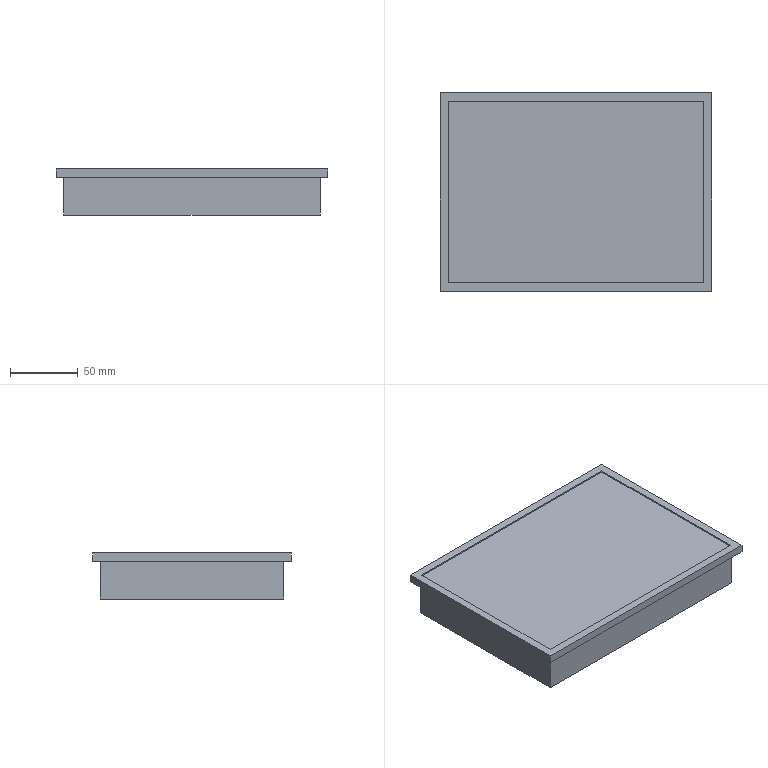Part | SolidWorks | features ICE 2, Extrusion 1 | 1 solid | 16 faces | box 200.3 x 146.3 x 34 mm | volume 870408 mm3 | plane 16
STEP:
#1=CARTESIAN_POINT('',(100.15,-73.15,0.));
#2=VERTEX_POINT('',#1);
#3=CARTESIAN_POINT('',(100.15,73.15,0.));
#4=VERTEX_POINT('',#3);
#5=CARTESIAN_POINT('',(100.15,73.15,0.));
#6=DIRECTION('',(0.,1.,0.));
#7=VECTOR('',#6,1000.);
#8=LINE('',#5,#7);
#9=EDGE_CURVE('',#2,#4,#8,.T.);
#10=ORIENTED_EDGE('',*,*,#9,.F.);
#11=CARTESIAN_POINT('',(-100.15,-73.15,0.));
#12=VERTEX_POINT('',#11);
#13=CARTESIAN_POINT('',(-100.15,-73.15,0.));
#14=DIRECTION('',(1.,0.,0.));
#15=VECTOR('',#14,1000.);
#16=LINE('',#13,#15);
#17=EDGE_CURVE('',#12,#2,#16,.T.);
#18=ORIENTED_EDGE('',*,*,#17,.F.);
#19=CARTESIAN_POINT('',(-100.15,73.15,0.));
#20=VERTEX_POINT('',#19);
#21=CARTESIAN_POINT('',(-100.15,73.15,0.));
#22=DIRECTION('',(0.,-1.,0.));
#23=VECTOR('',#22,1000.);
#24=LINE('',#21,#23);
#25=EDGE_CURVE('',#20,#12,#24,.T.);
#26=ORIENTED_EDGE('',*,*,#25,.F.);
#27=CARTESIAN_POINT('',(-100.15,73.15,0.));
#28=DIRECTION('',(-1.,0.,0.));
#29=VECTOR('',#28,1000.);
#30=LINE('',#27,#29);
#31=EDGE_CURVE('',#4,#20,#30,.T.);
#32=ORIENTED_EDGE('',*,*,#31,.F.);
#33=EDGE_LOOP('',(#10,#18,#26,#32));
#34=FACE_OUTER_BOUND('',#33,.T.);
#35=CARTESIAN_POINT('',(-94.8,-67.8,0.));
#36=VERTEX_POINT('',#35);
#37=CARTESIAN_POINT('',(-94.8,67.8,0.));
#38=VERTEX_POINT('',#37);
#39=CARTESIAN_POINT('',(-94.8,67.8,0.));
#40=DIRECTION('',(0.,1.,0.));
#41=VECTOR('',#40,1000.);
#42=LINE('',#39,#41);
#43=EDGE_CURVE('',#36,#38,#42,.T.);
#44=ORIENTED_EDGE('',*,*,#43,.F.);
#45=CARTESIAN_POINT('',(94.8,-67.8,0.));
#46=VERTEX_POINT('',#45);
#47=CARTESIAN_POINT('',(94.8,-67.8,0.));
#48=DIRECTION('',(-1.,0.,0.));
#49=VECTOR('',#48,1000.);
#50=LINE('',#47,#49);
#51=EDGE_CURVE('',#46,#36,#50,.T.);
#52=ORIENTED_EDGE('',*,*,#51,.F.);
#53=CARTESIAN_POINT('',(94.8,67.8,0.));
#54=VERTEX_POINT('',#53);
#55=CARTESIAN_POINT('',(94.8,67.8,0.));
#56=DIRECTION('',(0.,-1.,0.));
#57=VECTOR('',#56,1000.);
#58=LINE('',#55,#57);
#59=EDGE_CURVE('',#54,#46,#58,.T.);
#60=ORIENTED_EDGE('',*,*,#59,.F.);
#61=CARTESIAN_POINT('',(94.8,67.8,0.));
#62=DIRECTION('',(1.,0.,0.));
#63=VECTOR('',#62,1000.);
#64=LINE('',#61,#63);
#65=EDGE_CURVE('',#38,#54,#64,.T.);
#66=ORIENTED_EDGE('',*,*,#65,.F.);
#67=EDGE_LOOP('',(#44,#52,#60,#66));
#68=FACE_BOUND('',#67,.T.);
#69=CARTESIAN_POINT('',(0.,0.,0.));
#70=DIRECTION('',(0.,0.,1.));
#71=DIRECTION('',(1.,0.,0.));
#72=AXIS2_PLACEMENT_3D('',#69,#70,#71);
#73=PLANE('',#72);
#74=ADVANCED_FACE('',(#34,#68),#73,.F.);
#75=ORIENTED_EDGE('',*,*,#9,.T.);
#76=CARTESIAN_POINT('',(100.15,73.15,6.));
#77=VERTEX_POINT('',#76);
#78=CARTESIAN_POINT('',(100.15,73.15,6.));
#79=DIRECTION('',(0.,0.,-1.));
#80=VECTOR('',#79,1000.);
#81=LINE('',#78,#80);
#82=EDGE_CURVE('',#77,#4,#81,.T.);
#83=ORIENTED_EDGE('',*,*,#82,.F.);
#84=CARTESIAN_POINT('',(100.15,-73.15,6.));
#85=VERTEX_POINT('',#84);
#86=CARTESIAN_POINT('',(100.15,73.15,6.));
#87=DIRECTION('',(0.,1.,0.));
#88=VECTOR('',#87,1000.);
#89=LINE('',#86,#88);
#90=EDGE_CURVE('',#85,#77,#89,.T.);
#91=ORIENTED_EDGE('',*,*,#90,.F.);
#92=CARTESIAN_POINT('',(100.15,-73.15,6.));
#93=DIRECTION('',(0.,0.,-1.));
#94=VECTOR('',#93,1000.);
#95=LINE('',#92,#94);
#96=EDGE_CURVE('',#85,#2,#95,.T.);
#97=ORIENTED_EDGE('',*,*,#96,.T.);
#98=EDGE_LOOP('',(#75,#83,#91,#97));
#99=FACE_OUTER_BOUND('',#98,.T.);
#100=CARTESIAN_POINT('',(100.15,73.15,6.));
#101=DIRECTION('',(-1.,0.,0.));
#102=DIRECTION('',(0.,-1.,0.));
#103=AXIS2_PLACEMENT_3D('',#100,#101,#102);
#104=PLANE('',#103);
#105=ADVANCED_FACE('',(#99),#104,.F.);
#106=ORIENTED_EDGE('',*,*,#31,.T.);
#107=CARTESIAN_POINT('',(-100.15,73.15,6.));
#108=VERTEX_POINT('',#107);
#109=CARTESIAN_POINT('',(-100.15,73.15,6.));
#110=DIRECTION('',(0.,0.,-1.));
#111=VECTOR('',#110,1000.);
#112=LINE('',#109,#111);
#113=EDGE_CURVE('',#108,#20,#112,.T.);
#114=ORIENTED_EDGE('',*,*,#113,.F.);
#115=CARTESIAN_POINT('',(-100.15,73.15,6.));
#116=DIRECTION('',(-1.,0.,0.));
#117=VECTOR('',#116,1000.);
#118=LINE('',#115,#117);
#119=EDGE_CURVE('',#77,#108,#118,.T.);
#120=ORIENTED_EDGE('',*,*,#119,.F.);
#121=ORIENTED_EDGE('',*,*,#82,.T.);
#122=EDGE_LOOP('',(#106,#114,#120,#121));
#123=FACE_OUTER_BOUND('',#122,.T.);
#124=CARTESIAN_POINT('',(-100.15,73.15,6.));
#125=DIRECTION('',(0.,-1.,0.));
#126=DIRECTION('',(0.,0.,-1.));
#127=AXIS2_PLACEMENT_3D('',#124,#125,#126);
#128=PLANE('',#127);
#129=ADVANCED_FACE('',(#123),#128,.F.);
#130=ORIENTED_EDGE('',*,*,#25,.T.);
#131=CARTESIAN_POINT('',(-100.15,-73.15,6.));
#132=VERTEX_POINT('',#131);
#133=CARTESIAN_POINT('',(-100.15,-73.15,6.));
#134=DIRECTION('',(0.,0.,-1.));
#135=VECTOR('',#134,1000.);
#136=LINE('',#133,#135);
#137=EDGE_CURVE('',#132,#12,#136,.T.);
#138=ORIENTED_EDGE('',*,*,#137,.F.);
#139=CARTESIAN_POINT('',(-100.15,73.15,6.));
#140=DIRECTION('',(0.,-1.,0.));
#141=VECTOR('',#140,1000.);
#142=LINE('',#139,#141);
#143=EDGE_CURVE('',#108,#132,#142,.T.);
#144=ORIENTED_EDGE('',*,*,#143,.F.);
#145=ORIENTED_EDGE('',*,*,#113,.T.);
#146=EDGE_LOOP('',(#130,#138,#144,#145));
#147=FACE_OUTER_BOUND('',#146,.T.);
#148=CARTESIAN_POINT('',(-100.15,73.15,6.));
#149=DIRECTION('',(1.,0.,0.));
#150=DIRECTION('',(0.,0.,-1.));
#151=AXIS2_PLACEMENT_3D('',#148,#149,#150);
#152=PLANE('',#151);
#153=ADVANCED_FACE('',(#147),#152,.F.);
#154=ORIENTED_EDGE('',*,*,#17,.T.);
#155=ORIENTED_EDGE('',*,*,#96,.F.);
#156=CARTESIAN_POINT('',(-100.15,-73.15,6.));
#157=DIRECTION('',(1.,0.,0.));
#158=VECTOR('',#157,1000.);
#159=LINE('',#156,#158);
#160=EDGE_CURVE('',#132,#85,#159,.T.);
#161=ORIENTED_EDGE('',*,*,#160,.F.);
#162=ORIENTED_EDGE('',*,*,#137,.T.);
#163=EDGE_LOOP('',(#154,#155,#161,#162));
#164=FACE_OUTER_BOUND('',#163,.T.);
#165=CARTESIAN_POINT('',(-100.15,-73.15,6.));
#166=DIRECTION('',(0.,1.,0.));
#167=DIRECTION('',(0.,0.,1.));
#168=AXIS2_PLACEMENT_3D('',#165,#166,#167);
#169=PLANE('',#168);
#170=ADVANCED_FACE('',(#164),#169,.F.);
#171=CARTESIAN_POINT('',(94.15,-67.15,6.));
#172=VERTEX_POINT('',#171);
#173=CARTESIAN_POINT('',(94.15,67.15,6.));
#174=VERTEX_POINT('',#173);
#175=CARTESIAN_POINT('',(94.15,67.15,6.));
#176=DIRECTION('',(0.,1.,0.));
#177=VECTOR('',#176,1000.);
#178=LINE('',#175,#177);
#179=EDGE_CURVE('',#172,#174,#178,.T.);
#180=ORIENTED_EDGE('',*,*,#179,.F.);
#181=CARTESIAN_POINT('',(-94.15,-67.15,6.));
#182=VERTEX_POINT('',#181);
#183=CARTESIAN_POINT('',(-94.15,-67.15,6.));
#184=DIRECTION('',(1.,0.,0.));
#185=VECTOR('',#184,1000.);
#186=LINE('',#183,#185);
#187=EDGE_CURVE('',#182,#172,#186,.T.);
#188=ORIENTED_EDGE('',*,*,#187,.F.);
#189=CARTESIAN_POINT('',(-94.15,67.15,6.));
#190=VERTEX_POINT('',#189);
#191=CARTESIAN_POINT('',(-94.15,67.15,6.));
#192=DIRECTION('',(0.,-1.,0.));
#193=VECTOR('',#192,1000.);
#194=LINE('',#191,#193);
#195=EDGE_CURVE('',#190,#182,#194,.T.);
#196=ORIENTED_EDGE('',*,*,#195,.F.);
#197=CARTESIAN_POINT('',(-94.15,67.15,6.));
#198=DIRECTION('',(-1.,0.,0.));
#199=VECTOR('',#198,1000.);
#200=LINE('',#197,#199);
#201=EDGE_CURVE('',#174,#190,#200,.T.);
#202=ORIENTED_EDGE('',*,*,#201,.F.);
#203=EDGE_LOOP('',(#180,#188,#196,#202));
#204=FACE_BOUND('',#203,.T.);
#205=ORIENTED_EDGE('',*,*,#90,.T.);
#206=ORIENTED_EDGE('',*,*,#119,.T.);
#207=ORIENTED_EDGE('',*,*,#143,.T.);
#208=ORIENTED_EDGE('',*,*,#160,.T.);
#209=EDGE_LOOP('',(#205,#206,#207,#208));
#210=FACE_OUTER_BOUND('',#209,.T.);
#211=CARTESIAN_POINT('',(0.,0.,6.));
#212=DIRECTION('',(0.,0.,1.));
#213=DIRECTION('',(1.,0.,0.));
#214=AXIS2_PLACEMENT_3D('',#211,#212,#213);
#215=PLANE('',#214);
#216=ADVANCED_FACE('',(#204,#210),#215,.T.);
#217=ORIENTED_EDGE('',*,*,#43,.T.);
#218=CARTESIAN_POINT('',(-94.8,67.8,-28.));
#219=VERTEX_POINT('',#218);
#220=CARTESIAN_POINT('',(-94.8,67.8,-28.));
#221=DIRECTION('',(0.,0.,1.));
#222=VECTOR('',#221,1000.);
#223=LINE('',#220,#222);
#224=EDGE_CURVE('',#219,#38,#223,.T.);
#225=ORIENTED_EDGE('',*,*,#224,.F.);
#226=CARTESIAN_POINT('',(-94.8,-67.8,-28.));
#227=VERTEX_POINT('',#226);
#228=CARTESIAN_POINT('',(-94.8,67.8,-28.));
#229=DIRECTION('',(0.,1.,0.));
#230=VECTOR('',#229,1000.);
#231=LINE('',#228,#230);
#232=EDGE_CURVE('',#227,#219,#231,.T.);
#233=ORIENTED_EDGE('',*,*,#232,.F.);
#234=CARTESIAN_POINT('',(-94.8,-67.8,-28.));
#235=DIRECTION('',(0.,0.,1.));
#236=VECTOR('',#235,1000.);
#237=LINE('',#234,#236);
#238=EDGE_CURVE('',#227,#36,#237,.T.);
#239=ORIENTED_EDGE('',*,*,#238,.T.);
#240=EDGE_LOOP('',(#217,#225,#233,#239));
#241=FACE_OUTER_BOUND('',#240,.T.);
#242=CARTESIAN_POINT('',(-94.8,67.8,-28.));
#243=DIRECTION('',(1.,0.,0.));
#244=DIRECTION('',(0.,1.,0.));
#245=AXIS2_PLACEMENT_3D('',#242,#243,#244);
#246=PLANE('',#245);
#247=ADVANCED_FACE('',(#241),#246,.F.);
#248=ORIENTED_EDGE('',*,*,#65,.T.);
#249=CARTESIAN_POINT('',(94.8,67.8,-28.));
#250=VERTEX_POINT('',#249);
#251=CARTESIAN_POINT('',(94.8,67.8,-28.));
#252=DIRECTION('',(0.,0.,1.));
#253=VECTOR('',#252,1000.);
#254=LINE('',#251,#253);
#255=EDGE_CURVE('',#250,#54,#254,.T.);
#256=ORIENTED_EDGE('',*,*,#255,.F.);
#257=CARTESIAN_POINT('',(94.8,67.8,-28.));
#258=DIRECTION('',(1.,0.,0.));
#259=VECTOR('',#258,1000.);
#260=LINE('',#257,#259);
#261=EDGE_CURVE('',#219,#250,#260,.T.);
#262=ORIENTED_EDGE('',*,*,#261,.F.);
#263=ORIENTED_EDGE('',*,*,#224,.T.);
#264=EDGE_LOOP('',(#248,#256,#262,#263));
#265=FACE_OUTER_BOUND('',#264,.T.);
#266=CARTESIAN_POINT('',(94.8,67.8,-28.));
#267=DIRECTION('',(0.,-1.,0.));
#268=DIRECTION('',(0.,0.,-1.));
#269=AXIS2_PLACEMENT_3D('',#266,#267,#268);
#270=PLANE('',#269);
#271=ADVANCED_FACE('',(#265),#270,.F.);
#272=ORIENTED_EDGE('',*,*,#59,.T.);
#273=CARTESIAN_POINT('',(94.8,-67.8,-28.));
#274=VERTEX_POINT('',#273);
#275=CARTESIAN_POINT('',(94.8,-67.8,-28.));
#276=DIRECTION('',(0.,0.,1.));
#277=VECTOR('',#276,1000.);
#278=LINE('',#275,#277);
#279=EDGE_CURVE('',#274,#46,#278,.T.);
#280=ORIENTED_EDGE('',*,*,#279,.F.);
#281=CARTESIAN_POINT('',(94.8,67.8,-28.));
#282=DIRECTION('',(0.,-1.,0.));
#283=VECTOR('',#282,1000.);
#284=LINE('',#281,#283);
#285=EDGE_CURVE('',#250,#274,#284,.T.);
#286=ORIENTED_EDGE('',*,*,#285,.F.);
#287=ORIENTED_EDGE('',*,*,#255,.T.);
#288=EDGE_LOOP('',(#272,#280,#286,#287));
#289=FACE_OUTER_BOUND('',#288,.T.);
#290=CARTESIAN_POINT('',(94.8,67.8,-28.));
#291=DIRECTION('',(-1.,0.,0.));
#292=DIRECTION('',(0.,-1.,0.));
#293=AXIS2_PLACEMENT_3D('',#290,#291,#292);
#294=PLANE('',#293);
#295=ADVANCED_FACE('',(#289),#294,.F.);
#296=ORIENTED_EDGE('',*,*,#51,.T.);
#297=ORIENTED_EDGE('',*,*,#238,.F.);
#298=CARTESIAN_POINT('',(94.8,-67.8,-28.));
#299=DIRECTION('',(-1.,0.,0.));
#300=VECTOR('',#299,1000.);
#301=LINE('',#298,#300);
#302=EDGE_CURVE('',#274,#227,#301,.T.);
#303=ORIENTED_EDGE('',*,*,#302,.F.);
#304=ORIENTED_EDGE('',*,*,#279,.T.);
#305=EDGE_LOOP('',(#296,#297,#303,#304));
#306=FACE_OUTER_BOUND('',#305,.T.);
#307=CARTESIAN_POINT('',(94.8,-67.8,-28.));
#308=DIRECTION('',(0.,1.,0.));
#309=DIRECTION('',(0.,0.,1.));
#310=AXIS2_PLACEMENT_3D('',#307,#308,#309);
#311=PLANE('',#310);
#312=ADVANCED_FACE('',(#306),#311,.F.);
#313=ORIENTED_EDGE('',*,*,#232,.T.);
#314=ORIENTED_EDGE('',*,*,#261,.T.);
#315=ORIENTED_EDGE('',*,*,#285,.T.);
#316=ORIENTED_EDGE('',*,*,#302,.T.);
#317=EDGE_LOOP('',(#313,#314,#315,#316));
#318=FACE_OUTER_BOUND('',#317,.T.);
#319=CARTESIAN_POINT('',(0.,0.,-28.));
#320=DIRECTION('',(0.,0.,-1.));
#321=DIRECTION('',(-1.,0.,0.));
#322=AXIS2_PLACEMENT_3D('',#319,#320,#321);
#323=PLANE('',#322);
#324=ADVANCED_FACE('',(#318),#323,.T.);
#325=ORIENTED_EDGE('',*,*,#179,.T.);
#326=CARTESIAN_POINT('',(94.15,67.15,5.));
#327=VERTEX_POINT('',#326);
#328=CARTESIAN_POINT('',(94.15,67.15,5.));
#329=DIRECTION('',(0.,0.,1.));
#330=VECTOR('',#329,1000.);
#331=LINE('',#328,#330);
#332=EDGE_CURVE('',#327,#174,#331,.T.);
#333=ORIENTED_EDGE('',*,*,#332,.F.);
#334=CARTESIAN_POINT('',(94.15,-67.15,5.));
#335=VERTEX_POINT('',#334);
#336=CARTESIAN_POINT('',(94.15,67.15,5.));
#337=DIRECTION('',(0.,1.,0.));
#338=VECTOR('',#337,1000.);
#339=LINE('',#336,#338);
#340=EDGE_CURVE('',#335,#327,#339,.T.);
#341=ORIENTED_EDGE('',*,*,#340,.F.);
#342=CARTESIAN_POINT('',(94.15,-67.15,5.));
#343=DIRECTION('',(0.,0.,1.));
#344=VECTOR('',#343,1000.);
#345=LINE('',#342,#344);
#346=EDGE_CURVE('',#335,#172,#345,.T.);
#347=ORIENTED_EDGE('',*,*,#346,.T.);
#348=EDGE_LOOP('',(#325,#333,#341,#347));
#349=FACE_OUTER_BOUND('',#348,.T.);
#350=CARTESIAN_POINT('',(94.15,67.15,5.));
#351=DIRECTION('',(1.,0.,0.));
#352=DIRECTION('',(0.,0.,-1.));
#353=AXIS2_PLACEMENT_3D('',#350,#351,#352);
#354=PLANE('',#353);
#355=ADVANCED_FACE('',(#349),#354,.F.);
#356=ORIENTED_EDGE('',*,*,#187,.T.);
#357=ORIENTED_EDGE('',*,*,#346,.F.);
#358=CARTESIAN_POINT('',(-94.15,-67.15,5.));
#359=VERTEX_POINT('',#358);
#360=CARTESIAN_POINT('',(-94.15,-67.15,5.));
#361=DIRECTION('',(1.,0.,0.));
#362=VECTOR('',#361,1000.);
#363=LINE('',#360,#362);
#364=EDGE_CURVE('',#359,#335,#363,.T.);
#365=ORIENTED_EDGE('',*,*,#364,.F.);
#366=CARTESIAN_POINT('',(-94.15,-67.15,5.));
#367=DIRECTION('',(0.,0.,1.));
#368=VECTOR('',#367,1000.);
#369=LINE('',#366,#368);
#370=EDGE_CURVE('',#359,#182,#369,.T.);
#371=ORIENTED_EDGE('',*,*,#370,.T.);
#372=EDGE_LOOP('',(#356,#357,#365,#371));
#373=FACE_OUTER_BOUND('',#372,.T.);
#374=CARTESIAN_POINT('',(-94.15,-67.15,5.));
#375=DIRECTION('',(0.,-1.,0.));
#376=DIRECTION('',(0.,0.,-1.));
#377=AXIS2_PLACEMENT_3D('',#374,#375,#376);
#378=PLANE('',#377);
#379=ADVANCED_FACE('',(#373),#378,.F.);
#380=ORIENTED_EDGE('',*,*,#195,.T.);
#381=ORIENTED_EDGE('',*,*,#370,.F.);
#382=CARTESIAN_POINT('',(-94.15,67.15,5.));
#383=VERTEX_POINT('',#382);
#384=CARTESIAN_POINT('',(-94.15,67.15,5.));
#385=DIRECTION('',(0.,-1.,0.));
#386=VECTOR('',#385,1000.);
#387=LINE('',#384,#386);
#388=EDGE_CURVE('',#383,#359,#387,.T.);
#389=ORIENTED_EDGE('',*,*,#388,.F.);
#390=CARTESIAN_POINT('',(-94.15,67.15,5.));
#391=DIRECTION('',(0.,0.,1.));
#392=VECTOR('',#391,1000.);
#393=LINE('',#390,#392);
#394=EDGE_CURVE('',#383,#190,#393,.T.);
#395=ORIENTED_EDGE('',*,*,#394,.T.);
#396=EDGE_LOOP('',(#380,#381,#389,#395));
#397=FACE_OUTER_BOUND('',#396,.T.);
#398=CARTESIAN_POINT('',(-94.15,67.15,5.));
#399=DIRECTION('',(-1.,0.,0.));
#400=DIRECTION('',(0.,0.,1.));
#401=AXIS2_PLACEMENT_3D('',#398,#399,#400);
#402=PLANE('',#401);
#403=ADVANCED_FACE('',(#397),#402,.F.);
#404=ORIENTED_EDGE('',*,*,#201,.T.);
#405=ORIENTED_EDGE('',*,*,#394,.F.);
#406=CARTESIAN_POINT('',(-94.15,67.15,5.));
#407=DIRECTION('',(-1.,0.,0.));
#408=VECTOR('',#407,1000.);
#409=LINE('',#406,#408);
#410=EDGE_CURVE('',#327,#383,#409,.T.);
#411=ORIENTED_EDGE('',*,*,#410,.F.);
#412=ORIENTED_EDGE('',*,*,#332,.T.);
#413=EDGE_LOOP('',(#404,#405,#411,#412));
#414=FACE_OUTER_BOUND('',#413,.T.);
#415=CARTESIAN_POINT('',(-94.15,67.15,5.));
#416=DIRECTION('',(0.,1.,0.));
#417=DIRECTION('',(0.,0.,1.));
#418=AXIS2_PLACEMENT_3D('',#415,#416,#417);
#419=PLANE('',#418);
#420=ADVANCED_FACE('',(#414),#419,.F.);
#421=ORIENTED_EDGE('',*,*,#340,.T.);
#422=ORIENTED_EDGE('',*,*,#410,.T.);
#423=ORIENTED_EDGE('',*,*,#388,.T.);
#424=ORIENTED_EDGE('',*,*,#364,.T.);
#425=EDGE_LOOP('',(#421,#422,#423,#424));
#426=FACE_OUTER_BOUND('',#425,.T.);
#427=CARTESIAN_POINT('',(0.,0.,5.));
#428=DIRECTION('',(0.,0.,1.));
#429=DIRECTION('',(1.,0.,0.));
#430=AXIS2_PLACEMENT_3D('',#427,#428,#429);
#431=PLANE('',#430);
#432=ADVANCED_FACE('',(#426),#431,.T.);
#433=CLOSED_SHELL('',(#74,#105,#129,#153,#170,#216,#247,#271,#295,#312,#324,#355,#379,#403,#420,#432));
#434=MANIFOLD_SOLID_BREP('',#433);
#435=CARTESIAN_POINT('',(0.,0.,0.));
#436=DIRECTION('',(0.,0.,1.));
#437=DIRECTION('',(1.,0.,0.));
#438=AXIS2_PLACEMENT_3D('',#435,#436,#437);
#439=(LENGTH_UNIT()NAMED_UNIT(*)SI_UNIT(.MILLI.,.METRE.));
#440=UNCERTAINTY_MEASURE_WITH_UNIT(LENGTH_MEASURE(0.00001),#439,'','');
#441=(NAMED_UNIT(*)PLANE_ANGLE_UNIT()SI_UNIT($,.RADIAN.));
#442=(NAMED_UNIT(*)SI_UNIT($,.STERADIAN.)SOLID_ANGLE_UNIT());
#443=(GEOMETRIC_REPRESENTATION_CONTEXT(3)GLOBAL_UNCERTAINTY_ASSIGNED_CONTEXT((#440))GLOBAL_UNIT_ASSIGNED_CONTEXT((#439,#441,#442))REPRESENTATION_CONTEXT('',''));
#444=ADVANCED_BREP_SHAPE_REPRESENTATION('',(#434,#438),#443);